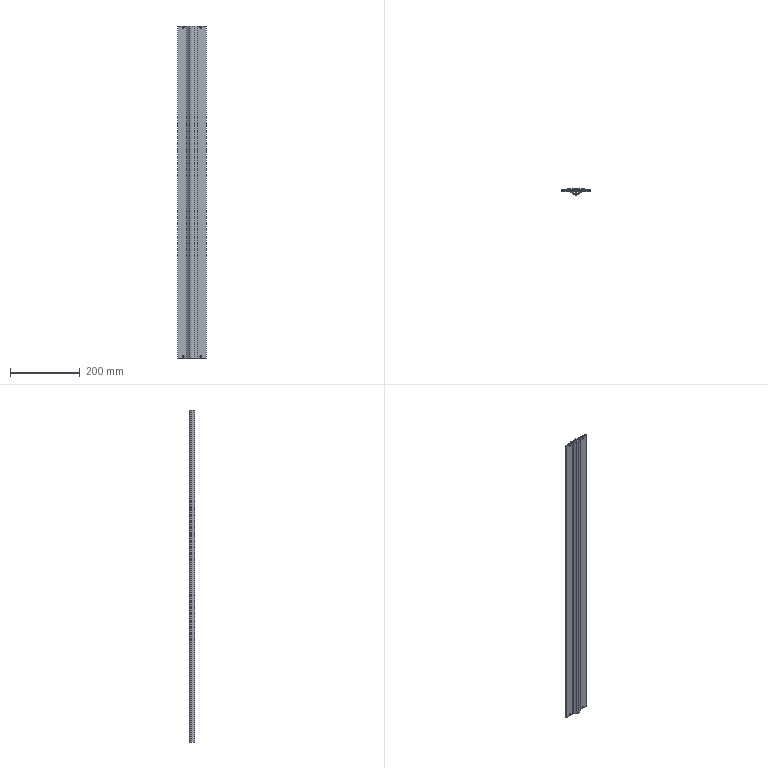Part | SolidWorks | features BaseBody 1 | 1 solid | 87 faces | box 82 x 17.089 x 949 mm | volume 309530 mm3 | cylinder 67 | plane 20 | commonest cylinder face diameters 0.6 x12 0.4 x10 4.5 x8 8 x8 1 x7 660 x7